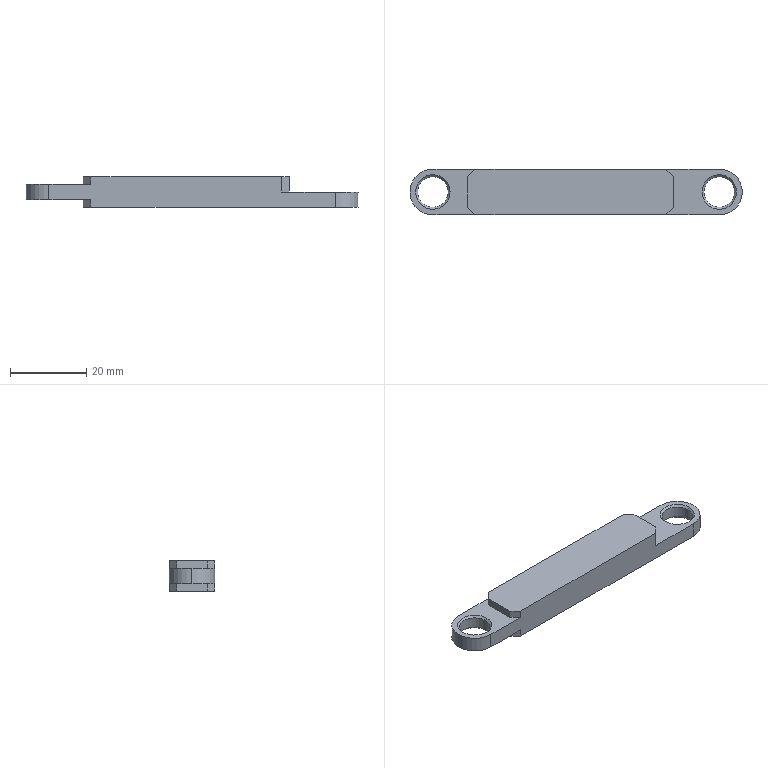Part | SolidWorks | features Chamfer 2, ICE 2, Extrusion 1 | 1 solid | 31 faces | box 87 x 12 x 8 mm | volume 6197 mm3 | plane 16 | cone 8 | cylinder 7 | commonest cylinder face diameters 8 x4 12 x3
STEP:
#1=CARTESIAN_POINT('',(33.5,0.,-0.5));
#2=VERTEX_POINT('',#1);
#3=CARTESIAN_POINT('',(41.5,0.,-0.5));
#4=VERTEX_POINT('',#3);
#5=CARTESIAN_POINT('',(37.5,0.,-0.5));
#6=DIRECTION('',(0.,0.,1.));
#7=DIRECTION('',(-1.,0.,0.));
#8=AXIS2_PLACEMENT_3D('',#5,#6,#7);
#9=CIRCLE('',#8,4.);
#10=EDGE_CURVE('',#2,#4,#9,.T.);
#11=ORIENTED_EDGE('',*,*,#10,.F.);
#12=CARTESIAN_POINT('',(33.,0.,0.));
#13=VERTEX_POINT('',#12);
#14=CARTESIAN_POINT('',(33.5,0.,-0.5));
#15=DIRECTION('',(-0.7071,0.,0.7071));
#16=VECTOR('',#15,1000.);
#17=LINE('',#14,#16);
#18=EDGE_CURVE('',#2,#13,#17,.T.);
#19=ORIENTED_EDGE('',*,*,#18,.T.);
#20=CARTESIAN_POINT('',(42.,0.,0.));
#21=VERTEX_POINT('',#20);
#22=CARTESIAN_POINT('',(37.5,0.,0.));
#23=DIRECTION('',(0.,0.,-1.));
#24=DIRECTION('',(-1.,0.,0.));
#25=AXIS2_PLACEMENT_3D('',#22,#23,#24);
#26=CIRCLE('',#25,4.5);
#27=EDGE_CURVE('',#21,#13,#26,.T.);
#28=ORIENTED_EDGE('',*,*,#27,.F.);
#29=CARTESIAN_POINT('',(41.5,0.,-0.5));
#30=DIRECTION('',(0.7071,0.,0.7071));
#31=VECTOR('',#30,1000.);
#32=LINE('',#29,#31);
#33=EDGE_CURVE('',#4,#21,#32,.T.);
#34=ORIENTED_EDGE('',*,*,#33,.F.);
#35=EDGE_LOOP('',(#11,#19,#28,#34));
#36=FACE_OUTER_BOUND('',#35,.T.);
#37=CARTESIAN_POINT('',(37.5,0.,-0.5));
#38=DIRECTION('',(0.,0.,1.));
#39=DIRECTION('',(1.,0.,0.));
#40=AXIS2_PLACEMENT_3D('',#37,#38,#39);
#41=CONICAL_SURFACE('',#40,4.,0.7854);
#42=ADVANCED_FACE('',(#36),#41,.F.);
#43=CARTESIAN_POINT('',(41.5,0.,-3.5));
#44=VERTEX_POINT('',#43);
#45=CARTESIAN_POINT('',(33.5,0.,-3.5));
#46=VERTEX_POINT('',#45);
#47=CARTESIAN_POINT('',(37.5,0.,-3.5));
#48=DIRECTION('',(0.,0.,-1.));
#49=DIRECTION('',(1.,0.,0.));
#50=AXIS2_PLACEMENT_3D('',#47,#48,#49);
#51=CIRCLE('',#50,4.);
#52=EDGE_CURVE('',#44,#46,#51,.T.);
#53=ORIENTED_EDGE('',*,*,#52,.F.);
#54=CARTESIAN_POINT('',(42.,0.,-4.));
#55=VERTEX_POINT('',#54);
#56=CARTESIAN_POINT('',(42.,0.,-4.));
#57=DIRECTION('',(0.7071,0.,-0.7071));
#58=VECTOR('',#57,1000.);
#59=LINE('',#56,#58);
#60=EDGE_CURVE('',#44,#55,#59,.T.);
#61=ORIENTED_EDGE('',*,*,#60,.T.);
#62=CARTESIAN_POINT('',(33.,0.,-4.));
#63=VERTEX_POINT('',#62);
#64=CARTESIAN_POINT('',(37.5,0.,-4.));
#65=DIRECTION('',(0.,0.,1.));
#66=DIRECTION('',(1.,0.,0.));
#67=AXIS2_PLACEMENT_3D('',#64,#65,#66);
#68=CIRCLE('',#67,4.5);
#69=EDGE_CURVE('',#63,#55,#68,.T.);
#70=ORIENTED_EDGE('',*,*,#69,.F.);
#71=CARTESIAN_POINT('',(33.,0.,-4.));
#72=DIRECTION('',(-0.7071,0.,-0.7071));
#73=VECTOR('',#72,1000.);
#74=LINE('',#71,#73);
#75=EDGE_CURVE('',#46,#63,#74,.T.);
#76=ORIENTED_EDGE('',*,*,#75,.F.);
#77=EDGE_LOOP('',(#53,#61,#70,#76));
#78=FACE_OUTER_BOUND('',#77,.T.);
#79=CARTESIAN_POINT('',(37.5,0.,-4.));
#80=DIRECTION('',(0.,0.,-1.));
#81=DIRECTION('',(-1.,0.,0.));
#82=AXIS2_PLACEMENT_3D('',#79,#80,#81);
#83=CONICAL_SURFACE('',#82,4.5,0.7854);
#84=ADVANCED_FACE('',(#78),#83,.F.);
#85=CARTESIAN_POINT('',(-41.5,0.,1.5));
#86=VERTEX_POINT('',#85);
#87=CARTESIAN_POINT('',(-33.5,0.,1.5));
#88=VERTEX_POINT('',#87);
#89=CARTESIAN_POINT('',(-37.5,0.,1.5));
#90=DIRECTION('',(0.,0.,1.));
#91=DIRECTION('',(-1.,0.,0.));
#92=AXIS2_PLACEMENT_3D('',#89,#90,#91);
#93=CIRCLE('',#92,4.);
#94=EDGE_CURVE('',#86,#88,#93,.T.);
#95=ORIENTED_EDGE('',*,*,#94,.F.);
#96=CARTESIAN_POINT('',(-42.,0.,2.));
#97=VERTEX_POINT('',#96);
#98=CARTESIAN_POINT('',(-41.5,0.,1.5));
#99=DIRECTION('',(-0.7071,0.,0.7071));
#100=VECTOR('',#99,1000.);
#101=LINE('',#98,#100);
#102=EDGE_CURVE('',#86,#97,#101,.T.);
#103=ORIENTED_EDGE('',*,*,#102,.T.);
#104=CARTESIAN_POINT('',(-33.,0.,2.));
#105=VERTEX_POINT('',#104);
#106=CARTESIAN_POINT('',(-37.5,0.,2.));
#107=DIRECTION('',(0.,0.,-1.));
#108=DIRECTION('',(-1.,0.,0.));
#109=AXIS2_PLACEMENT_3D('',#106,#107,#108);
#110=CIRCLE('',#109,4.5);
#111=EDGE_CURVE('',#105,#97,#110,.T.);
#112=ORIENTED_EDGE('',*,*,#111,.F.);
#113=CARTESIAN_POINT('',(-33.5,0.,1.5));
#114=DIRECTION('',(0.7071,0.,0.7071));
#115=VECTOR('',#114,1000.);
#116=LINE('',#113,#115);
#117=EDGE_CURVE('',#88,#105,#116,.T.);
#118=ORIENTED_EDGE('',*,*,#117,.F.);
#119=EDGE_LOOP('',(#95,#103,#112,#118));
#120=FACE_OUTER_BOUND('',#119,.T.);
#121=CARTESIAN_POINT('',(-37.5,0.,1.5));
#122=DIRECTION('',(0.,0.,1.));
#123=DIRECTION('',(1.,0.,0.));
#124=AXIS2_PLACEMENT_3D('',#121,#122,#123);
#125=CONICAL_SURFACE('',#124,4.,0.7854);
#126=ADVANCED_FACE('',(#120),#125,.F.);
#127=CARTESIAN_POINT('',(-33.5,0.,-1.5));
#128=VERTEX_POINT('',#127);
#129=CARTESIAN_POINT('',(-41.5,0.,-1.5));
#130=VERTEX_POINT('',#129);
#131=CARTESIAN_POINT('',(-37.5,0.,-1.5));
#132=DIRECTION('',(0.,0.,-1.));
#133=DIRECTION('',(1.,0.,0.));
#134=AXIS2_PLACEMENT_3D('',#131,#132,#133);
#135=CIRCLE('',#134,4.);
#136=EDGE_CURVE('',#128,#130,#135,.T.);
#137=ORIENTED_EDGE('',*,*,#136,.F.);
#138=CARTESIAN_POINT('',(-33.,0.,-2.));
#139=VERTEX_POINT('',#138);
#140=CARTESIAN_POINT('',(-33.5,0.,-1.5));
#141=DIRECTION('',(0.7071,0.,-0.7071));
#142=VECTOR('',#141,1000.);
#143=LINE('',#140,#142);
#144=EDGE_CURVE('',#128,#139,#143,.T.);
#145=ORIENTED_EDGE('',*,*,#144,.T.);
#146=CARTESIAN_POINT('',(-42.,0.,-2.));
#147=VERTEX_POINT('',#146);
#148=CARTESIAN_POINT('',(-37.5,0.,-2.));
#149=DIRECTION('',(0.,0.,1.));
#150=DIRECTION('',(1.,0.,0.));
#151=AXIS2_PLACEMENT_3D('',#148,#149,#150);
#152=CIRCLE('',#151,4.5);
#153=EDGE_CURVE('',#147,#139,#152,.T.);
#154=ORIENTED_EDGE('',*,*,#153,.F.);
#155=CARTESIAN_POINT('',(-41.5,0.,-1.5));
#156=DIRECTION('',(-0.7071,0.,-0.7071));
#157=VECTOR('',#156,1000.);
#158=LINE('',#155,#157);
#159=EDGE_CURVE('',#130,#147,#158,.T.);
#160=ORIENTED_EDGE('',*,*,#159,.F.);
#161=EDGE_LOOP('',(#137,#145,#154,#160));
#162=FACE_OUTER_BOUND('',#161,.T.);
#163=CARTESIAN_POINT('',(-37.5,0.,-1.5));
#164=DIRECTION('',(0.,0.,-1.));
#165=DIRECTION('',(-1.,0.,0.));
#166=AXIS2_PLACEMENT_3D('',#163,#164,#165);
#167=CONICAL_SURFACE('',#166,4.,0.7854);
#168=ADVANCED_FACE('',(#162),#167,.F.);
#169=ORIENTED_EDGE('',*,*,#136,.T.);
#170=CARTESIAN_POINT('',(-41.5,0.,-4.));
#171=DIRECTION('',(0.,0.,1.));
#172=VECTOR('',#171,1000.);
#173=LINE('',#170,#172);
#174=EDGE_CURVE('',#130,#86,#173,.T.);
#175=ORIENTED_EDGE('',*,*,#174,.T.);
#176=ORIENTED_EDGE('',*,*,#94,.T.);
#177=CARTESIAN_POINT('',(-33.5,0.,-4.));
#178=DIRECTION('',(0.,0.,1.));
#179=VECTOR('',#178,1000.);
#180=LINE('',#177,#179);
#181=EDGE_CURVE('',#128,#88,#180,.T.);
#182=ORIENTED_EDGE('',*,*,#181,.F.);
#183=EDGE_LOOP('',(#169,#175,#176,#182));
#184=FACE_OUTER_BOUND('',#183,.T.);
#185=CARTESIAN_POINT('',(-37.5,0.,-4.));
#186=DIRECTION('',(0.,0.,1.));
#187=DIRECTION('',(1.,0.,0.));
#188=AXIS2_PLACEMENT_3D('',#185,#186,#187);
#189=CYLINDRICAL_SURFACE('',#188,4.);
#190=ADVANCED_FACE('',(#184),#189,.F.);
#191=ORIENTED_EDGE('',*,*,#52,.T.);
#192=CARTESIAN_POINT('',(33.5,0.,-4.));
#193=DIRECTION('',(0.,0.,1.));
#194=VECTOR('',#193,1000.);
#195=LINE('',#192,#194);
#196=EDGE_CURVE('',#46,#2,#195,.T.);
#197=ORIENTED_EDGE('',*,*,#196,.T.);
#198=ORIENTED_EDGE('',*,*,#10,.T.);
#199=CARTESIAN_POINT('',(41.5,0.,-4.));
#200=DIRECTION('',(0.,0.,1.));
#201=VECTOR('',#200,1000.);
#202=LINE('',#199,#201);
#203=EDGE_CURVE('',#44,#4,#202,.T.);
#204=ORIENTED_EDGE('',*,*,#203,.F.);
#205=EDGE_LOOP('',(#191,#197,#198,#204));
#206=FACE_OUTER_BOUND('',#205,.T.);
#207=CARTESIAN_POINT('',(37.5,0.,-4.));
#208=DIRECTION('',(0.,0.,1.));
#209=DIRECTION('',(1.,0.,0.));
#210=AXIS2_PLACEMENT_3D('',#207,#208,#209);
#211=CYLINDRICAL_SURFACE('',#210,4.);
#212=ADVANCED_FACE('',(#206),#211,.F.);
#213=CARTESIAN_POINT('',(-37.5,-6.,2.));
#214=VERTEX_POINT('',#213);
#215=CARTESIAN_POINT('',(-43.5,0.,2.));
#216=VERTEX_POINT('',#215);
#217=CARTESIAN_POINT('',(-37.5,0.,2.));
#218=DIRECTION('',(0.,0.,-1.));
#219=DIRECTION('',(-1.,0.,0.));
#220=AXIS2_PLACEMENT_3D('',#217,#218,#219);
#221=CIRCLE('',#220,6.);
#222=EDGE_CURVE('',#214,#216,#221,.T.);
#223=ORIENTED_EDGE('',*,*,#222,.T.);
#224=CARTESIAN_POINT('',(-43.5,0.,-2.));
#225=VERTEX_POINT('',#224);
#226=CARTESIAN_POINT('',(-43.5,0.,4.));
#227=DIRECTION('',(0.,0.,-1.));
#228=VECTOR('',#227,1000.);
#229=LINE('',#226,#228);
#230=EDGE_CURVE('',#216,#225,#229,.T.);
#231=ORIENTED_EDGE('',*,*,#230,.T.);
#232=CARTESIAN_POINT('',(-37.5,-6.,-2.));
#233=VERTEX_POINT('',#232);
#234=CARTESIAN_POINT('',(-37.5,0.,-2.));
#235=DIRECTION('',(0.,0.,1.));
#236=DIRECTION('',(1.,0.,0.));
#237=AXIS2_PLACEMENT_3D('',#234,#235,#236);
#238=CIRCLE('',#237,6.);
#239=EDGE_CURVE('',#225,#233,#238,.T.);
#240=ORIENTED_EDGE('',*,*,#239,.T.);
#241=CARTESIAN_POINT('',(-37.5,-6.,4.));
#242=DIRECTION('',(0.,0.,-1.));
#243=VECTOR('',#242,1000.);
#244=LINE('',#241,#243);
#245=EDGE_CURVE('',#214,#233,#244,.T.);
#246=ORIENTED_EDGE('',*,*,#245,.F.);
#247=EDGE_LOOP('',(#223,#231,#240,#246));
#248=FACE_OUTER_BOUND('',#247,.T.);
#249=CARTESIAN_POINT('',(-37.5,0.,4.));
#250=DIRECTION('',(0.,0.,-1.));
#251=DIRECTION('',(-1.,0.,0.));
#252=AXIS2_PLACEMENT_3D('',#249,#250,#251);
#253=CYLINDRICAL_SURFACE('',#252,6.);
#254=ADVANCED_FACE('',(#248),#253,.T.);
#255=ORIENTED_EDGE('',*,*,#230,.F.);
#256=CARTESIAN_POINT('',(-37.5,6.,2.));
#257=VERTEX_POINT('',#256);
#258=CARTESIAN_POINT('',(-37.5,0.,2.));
#259=DIRECTION('',(0.,0.,-1.));
#260=DIRECTION('',(-1.,0.,0.));
#261=AXIS2_PLACEMENT_3D('',#258,#259,#260);
#262=CIRCLE('',#261,6.);
#263=EDGE_CURVE('',#216,#257,#262,.T.);
#264=ORIENTED_EDGE('',*,*,#263,.T.);
#265=CARTESIAN_POINT('',(-37.5,6.,-2.));
#266=VERTEX_POINT('',#265);
#267=CARTESIAN_POINT('',(-37.5,6.,4.));
#268=DIRECTION('',(0.,0.,-1.));
#269=VECTOR('',#268,1000.);
#270=LINE('',#267,#269);
#271=EDGE_CURVE('',#257,#266,#270,.T.);
#272=ORIENTED_EDGE('',*,*,#271,.T.);
#273=CARTESIAN_POINT('',(-37.5,0.,-2.));
#274=DIRECTION('',(0.,0.,1.));
#275=DIRECTION('',(1.,0.,0.));
#276=AXIS2_PLACEMENT_3D('',#273,#274,#275);
#277=CIRCLE('',#276,6.);
#278=EDGE_CURVE('',#266,#225,#277,.T.);
#279=ORIENTED_EDGE('',*,*,#278,.T.);
#280=EDGE_LOOP('',(#255,#264,#272,#279));
#281=FACE_OUTER_BOUND('',#280,.T.);
#282=CARTESIAN_POINT('',(-37.5,0.,4.));
#283=DIRECTION('',(0.,0.,-1.));
#284=DIRECTION('',(-1.,0.,0.));
#285=AXIS2_PLACEMENT_3D('',#282,#283,#284);
#286=CYLINDRICAL_SURFACE('',#285,6.);
#287=ADVANCED_FACE('',(#281),#286,.T.);
#288=CARTESIAN_POINT('',(-26.5,-6.,-2.));
#289=VERTEX_POINT('',#288);
#290=CARTESIAN_POINT('',(-43.5,-6.,-2.));
#291=DIRECTION('',(1.,0.,0.));
#292=VECTOR('',#291,1000.);
#293=LINE('',#290,#292);
#294=EDGE_CURVE('',#233,#289,#293,.T.);
#295=ORIENTED_EDGE('',*,*,#294,.T.);
#296=CARTESIAN_POINT('',(-26.5,-6.,-4.));
#297=VERTEX_POINT('',#296);
#298=CARTESIAN_POINT('',(-26.5,-6.,4.));
#299=DIRECTION('',(0.,0.,-1.));
#300=VECTOR('',#299,1000.);
#301=LINE('',#298,#300);
#302=EDGE_CURVE('',#289,#297,#301,.T.);
#303=ORIENTED_EDGE('',*,*,#302,.T.);
#304=CARTESIAN_POINT('',(37.5,-6.,-4.));
#305=VERTEX_POINT('',#304);
#306=CARTESIAN_POINT('',(-37.5,-6.,-4.));
#307=DIRECTION('',(1.,0.,0.));
#308=VECTOR('',#307,1000.);
#309=LINE('',#306,#308);
#310=EDGE_CURVE('',#297,#305,#309,.T.);
#311=ORIENTED_EDGE('',*,*,#310,.T.);
#312=CARTESIAN_POINT('',(37.5,-6.,0.));
#313=VERTEX_POINT('',#312);
#314=CARTESIAN_POINT('',(37.5,-6.,4.));
#315=DIRECTION('',(0.,0.,-1.));
#316=VECTOR('',#315,1000.);
#317=LINE('',#314,#316);
#318=EDGE_CURVE('',#313,#305,#317,.T.);
#319=ORIENTED_EDGE('',*,*,#318,.F.);
#320=CARTESIAN_POINT('',(23.5,-6.,0.));
#321=VERTEX_POINT('',#320);
#322=CARTESIAN_POINT('',(25.5,-6.,0.));
#323=DIRECTION('',(-1.,0.,0.));
#324=VECTOR('',#323,1000.);
#325=LINE('',#322,#324);
#326=EDGE_CURVE('',#313,#321,#325,.T.);
#327=ORIENTED_EDGE('',*,*,#326,.T.);
#328=CARTESIAN_POINT('',(23.5,-6.,4.));
#329=VERTEX_POINT('',#328);
#330=CARTESIAN_POINT('',(23.5,-6.,4.));
#331=DIRECTION('',(0.,0.,1.));
#332=VECTOR('',#331,1000.);
#333=LINE('',#330,#332);
#334=EDGE_CURVE('',#321,#329,#333,.T.);
#335=ORIENTED_EDGE('',*,*,#334,.T.);
#336=CARTESIAN_POINT('',(-26.5,-6.,4.));
#337=VERTEX_POINT('',#336);
#338=CARTESIAN_POINT('',(-37.5,-6.,4.));
#339=DIRECTION('',(1.,0.,0.));
#340=VECTOR('',#339,1000.);
#341=LINE('',#338,#340);
#342=EDGE_CURVE('',#337,#329,#341,.T.);
#343=ORIENTED_EDGE('',*,*,#342,.F.);
#344=CARTESIAN_POINT('',(-26.5,-6.,2.));
#345=VERTEX_POINT('',#344);
#346=CARTESIAN_POINT('',(-26.5,-6.,4.));
#347=DIRECTION('',(0.,0.,-1.));
#348=VECTOR('',#347,1000.);
#349=LINE('',#346,#348);
#350=EDGE_CURVE('',#337,#345,#349,.T.);
#351=ORIENTED_EDGE('',*,*,#350,.T.);
#352=CARTESIAN_POINT('',(-43.5,-6.,2.));
#353=DIRECTION('',(-1.,0.,0.));
#354=VECTOR('',#353,1000.);
#355=LINE('',#352,#354);
#356=EDGE_CURVE('',#345,#214,#355,.T.);
#357=ORIENTED_EDGE('',*,*,#356,.T.);
#358=ORIENTED_EDGE('',*,*,#245,.T.);
#359=EDGE_LOOP('',(#295,#303,#311,#319,#327,#335,#343,#351,#357,#358));
#360=FACE_OUTER_BOUND('',#359,.T.);
#361=CARTESIAN_POINT('',(-37.5,-6.,4.));
#362=DIRECTION('',(0.,1.,0.));
#363=DIRECTION('',(0.,0.,1.));
#364=AXIS2_PLACEMENT_3D('',#361,#362,#363);
#365=PLANE('',#364);
#366=ADVANCED_FACE('',(#360),#365,.F.);
#367=CARTESIAN_POINT('',(37.5,6.,0.));
#368=VERTEX_POINT('',#367);
#369=CARTESIAN_POINT('',(37.5,6.,-4.));
#370=VERTEX_POINT('',#369);
#371=CARTESIAN_POINT('',(37.5,6.,4.));
#372=DIRECTION('',(0.,0.,-1.));
#373=VECTOR('',#372,1000.);
#374=LINE('',#371,#373);
#375=EDGE_CURVE('',#368,#370,#374,.T.);
#376=ORIENTED_EDGE('',*,*,#375,.F.);
#377=CARTESIAN_POINT('',(37.5,0.,0.));
#378=DIRECTION('',(0.,0.,-1.));
#379=DIRECTION('',(-1.,0.,0.));
#380=AXIS2_PLACEMENT_3D('',#377,#378,#379);
#381=CIRCLE('',#380,6.);
#382=EDGE_CURVE('',#368,#313,#381,.T.);
#383=ORIENTED_EDGE('',*,*,#382,.T.);
#384=ORIENTED_EDGE('',*,*,#318,.T.);
#385=CARTESIAN_POINT('',(37.5,0.,-4.));
#386=DIRECTION('',(0.,0.,1.));
#387=DIRECTION('',(1.,0.,0.));
#388=AXIS2_PLACEMENT_3D('',#385,#386,#387);
#389=CIRCLE('',#388,6.);
#390=EDGE_CURVE('',#305,#370,#389,.T.);
#391=ORIENTED_EDGE('',*,*,#390,.T.);
#392=EDGE_LOOP('',(#376,#383,#384,#391));
#393=FACE_OUTER_BOUND('',#392,.T.);
#394=CARTESIAN_POINT('',(37.5,0.,4.));
#395=DIRECTION('',(0.,0.,-1.));
#396=DIRECTION('',(-1.,0.,0.));
#397=AXIS2_PLACEMENT_3D('',#394,#395,#396);
#398=CYLINDRICAL_SURFACE('',#397,6.);
#399=ADVANCED_FACE('',(#393),#398,.T.);
#400=CARTESIAN_POINT('',(-26.5,6.,-4.));
#401=VERTEX_POINT('',#400);
#402=CARTESIAN_POINT('',(-37.5,6.,-4.));
#403=DIRECTION('',(-1.,0.,0.));
#404=VECTOR('',#403,1000.);
#405=LINE('',#402,#404);
#406=EDGE_CURVE('',#370,#401,#405,.T.);
#407=ORIENTED_EDGE('',*,*,#406,.T.);
#408=CARTESIAN_POINT('',(-26.5,6.,-2.));
#409=VERTEX_POINT('',#408);
#410=CARTESIAN_POINT('',(-26.5,6.,4.));
#411=DIRECTION('',(0.,0.,1.));
#412=VECTOR('',#411,1000.);
#413=LINE('',#410,#412);
#414=EDGE_CURVE('',#401,#409,#413,.T.);
#415=ORIENTED_EDGE('',*,*,#414,.T.);
#416=CARTESIAN_POINT('',(-43.5,6.,-2.));
#417=DIRECTION('',(1.,0.,0.));
#418=VECTOR('',#417,1000.);
#419=LINE('',#416,#418);
#420=EDGE_CURVE('',#266,#409,#419,.T.);
#421=ORIENTED_EDGE('',*,*,#420,.F.);
#422=ORIENTED_EDGE('',*,*,#271,.F.);
#423=CARTESIAN_POINT('',(-26.5,6.,2.));
#424=VERTEX_POINT('',#423);
#425=CARTESIAN_POINT('',(-43.5,6.,2.));
#426=DIRECTION('',(-1.,0.,0.));
#427=VECTOR('',#426,1000.);
#428=LINE('',#425,#427);
#429=EDGE_CURVE('',#424,#257,#428,.T.);
#430=ORIENTED_EDGE('',*,*,#429,.F.);
#431=CARTESIAN_POINT('',(-26.5,6.,4.));
#432=VERTEX_POINT('',#431);
#433=CARTESIAN_POINT('',(-26.5,6.,4.));
#434=DIRECTION('',(0.,0.,1.));
#435=VECTOR('',#434,1000.);
#436=LINE('',#433,#435);
#437=EDGE_CURVE('',#424,#432,#436,.T.);
#438=ORIENTED_EDGE('',*,*,#437,.T.);
#439=CARTESIAN_POINT('',(23.5,6.,4.));
#440=VERTEX_POINT('',#439);
#441=CARTESIAN_POINT('',(-37.5,6.,4.));
#442=DIRECTION('',(-1.,0.,0.));
#443=VECTOR('',#442,1000.);
#444=LINE('',#441,#443);
#445=EDGE_CURVE('',#440,#432,#444,.T.);
#446=ORIENTED_EDGE('',*,*,#445,.F.);
#447=CARTESIAN_POINT('',(23.5,6.,0.));
#448=VERTEX_POINT('',#447);
#449=CARTESIAN_POINT('',(23.5,6.,4.));
#450=DIRECTION('',(0.,0.,-1.));
#451=VECTOR('',#450,1000.);
#452=LINE('',#449,#451);
#453=EDGE_CURVE('',#440,#448,#452,.T.);
#454=ORIENTED_EDGE('',*,*,#453,.T.);
#455=CARTESIAN_POINT('',(25.5,6.,0.));
#456=DIRECTION('',(-1.,0.,0.));
#457=VECTOR('',#456,1000.);
#458=LINE('',#455,#457);
#459=EDGE_CURVE('',#368,#448,#458,.T.);
#460=ORIENTED_EDGE('',*,*,#459,.F.);
#461=ORIENTED_EDGE('',*,*,#375,.T.);
#462=EDGE_LOOP('',(#407,#415,#421,#422,#430,#438,#446,#454,#460,#461));
#463=FACE_OUTER_BOUND('',#462,.T.);
#464=CARTESIAN_POINT('',(-37.5,6.,4.));
#465=DIRECTION('',(0.,-1.,0.));
#466=DIRECTION('',(0.,0.,-1.));
#467=AXIS2_PLACEMENT_3D('',#464,#465,#466);
#468=PLANE('',#467);
#469=ADVANCED_FACE('',(#463),#468,.F.);
#470=ORIENTED_EDGE('',*,*,#445,.T.);
#471=CARTESIAN_POINT('',(-28.5,4.,4.));
#472=VERTEX_POINT('',#471);
#473=CARTESIAN_POINT('',(-35.,-2.5,4.));
#474=DIRECTION('',(-0.7071,-0.7071,0.));
#475=VECTOR('',#474,1000.);
#476=LINE('',#473,#475);
#477=EDGE_CURVE('',#432,#472,#476,.T.);
#478=ORIENTED_EDGE('',*,*,#477,.T.);
#479=CARTESIAN_POINT('',(-28.5,-4.,4.));
#480=VERTEX_POINT('',#479);
#481=CARTESIAN_POINT('',(-28.5,-6.,4.));
#482=DIRECTION('',(0.,1.,0.));
#483=VECTOR('',#482,1000.);
#484=LINE('',#481,#483);
#485=EDGE_CURVE('',#480,#472,#484,.T.);
#486=ORIENTED_EDGE('',*,*,#485,.F.);
#487=CARTESIAN_POINT('',(-35.,2.5,4.));
#488=DIRECTION('',(0.7071,-0.7071,0.));
#489=VECTOR('',#488,1000.);
#490=LINE('',#487,#489);
#491=EDGE_CURVE('',#480,#337,#490,.T.);
#492=ORIENTED_EDGE('',*,*,#491,.T.);
#493=ORIENTED_EDGE('',*,*,#342,.T.);
#494=CARTESIAN_POINT('',(25.5,-4.,4.));
#495=VERTEX_POINT('',#494);
#496=CARTESIAN_POINT('',(-4.,-33.5,4.));
#497=DIRECTION('',(0.7071,0.7071,0.));
#498=VECTOR('',#497,1000.);
#499=LINE('',#496,#498);
#500=EDGE_CURVE('',#329,#495,#499,.T.);
#501=ORIENTED_EDGE('',*,*,#500,.T.);
#502=CARTESIAN_POINT('',(25.5,4.,4.));
#503=VERTEX_POINT('',#502);
#504=CARTESIAN_POINT('',(25.5,-6.,4.));
#505=DIRECTION('',(0.,1.,0.));
#506=VECTOR('',#505,1000.);
#507=LINE('',#504,#506);
#508=EDGE_CURVE('',#495,#503,#507,.T.);
#509=ORIENTED_EDGE('',*,*,#508,.T.);
#510=CARTESIAN_POINT('',(-4.,33.5,4.));
#511=DIRECTION('',(-0.7071,0.7071,0.));
#512=VECTOR('',#511,1000.);
#513=LINE('',#510,#512);
#514=EDGE_CURVE('',#503,#440,#513,.T.);
#515=ORIENTED_EDGE('',*,*,#514,.T.);
#516=EDGE_LOOP('',(#470,#478,#486,#492,#493,#501,#509,#515));
#517=FACE_OUTER_BOUND('',#516,.T.);
#518=CARTESIAN_POINT('',(-37.5,0.,4.));
#519=DIRECTION('',(0.,0.,1.));
#520=DIRECTION('',(1.,0.,0.));
#521=AXIS2_PLACEMENT_3D('',#518,#519,#520);
#522=PLANE('',#521);
#523=ADVANCED_FACE('',(#517),#522,.T.);
#524=ORIENTED_EDGE('',*,*,#69,.T.);
#525=CARTESIAN_POINT('',(37.5,0.,-4.));
#526=DIRECTION('',(0.,0.,1.));
#527=DIRECTION('',(1.,0.,0.));
#528=AXIS2_PLACEMENT_3D('',#525,#526,#527);
#529=CIRCLE('',#528,4.5);
#530=EDGE_CURVE('',#55,#63,#529,.T.);
#531=ORIENTED_EDGE('',*,*,#530,.T.);
#532=EDGE_LOOP('',(#524,#531));
#533=FACE_BOUND('',#532,.T.);
#534=CARTESIAN_POINT('',(-28.5,-4.,-4.));
#535=VERTEX_POINT('',#534);
#536=CARTESIAN_POINT('',(-28.5,4.,-4.));
#537=VERTEX_POINT('',#536);
#538=CARTESIAN_POINT('',(-28.5,-6.,-4.));
#539=DIRECTION('',(0.,1.,0.));
#540=VECTOR('',#539,1000.);
#541=LINE('',#538,#540);
#542=EDGE_CURVE('',#535,#537,#541,.T.);
#543=ORIENTED_EDGE('',*,*,#542,.T.);
#544=CARTESIAN_POINT('',(-28.5,4.,-4.));
#545=DIRECTION('',(0.7071,0.7071,0.));
#546=VECTOR('',#545,1000.);
#547=LINE('',#544,#546);
#548=EDGE_CURVE('',#537,#401,#547,.T.);
#549=ORIENTED_EDGE('',*,*,#548,.T.);
#550=ORIENTED_EDGE('',*,*,#406,.F.);
#551=ORIENTED_EDGE('',*,*,#390,.F.);
#552=ORIENTED_EDGE('',*,*,#310,.F.);
#553=CARTESIAN_POINT('',(-26.5,-6.,-4.));
#554=DIRECTION('',(-0.7071,0.7071,0.));
#555=VECTOR('',#554,1000.);
#556=LINE('',#553,#555);
#557=EDGE_CURVE('',#297,#535,#556,.T.);
#558=ORIENTED_EDGE('',*,*,#557,.T.);
#559=EDGE_LOOP('',(#543,#549,#550,#551,#552,#558));
#560=FACE_OUTER_BOUND('',#559,.T.);
#561=CARTESIAN_POINT('',(-37.5,0.,-4.));
#562=DIRECTION('',(0.,0.,1.));
#563=DIRECTION('',(1.,0.,0.));
#564=AXIS2_PLACEMENT_3D('',#561,#562,#563);
#565=PLANE('',#564);
#566=ADVANCED_FACE('',(#533,#560),#565,.F.);
#567=ORIENTED_EDGE('',*,*,#196,.F.);
#568=CARTESIAN_POINT('',(37.5,0.,-3.5));
#569=DIRECTION('',(0.,0.,-1.));
#570=DIRECTION('',(1.,0.,0.));
#571=AXIS2_PLACEMENT_3D('',#568,#569,#570);
#572=CIRCLE('',#571,4.);
#573=EDGE_CURVE('',#46,#44,#572,.T.);
#574=ORIENTED_EDGE('',*,*,#573,.T.);
#575=ORIENTED_EDGE('',*,*,#203,.T.);
#576=CARTESIAN_POINT('',(37.5,0.,-0.5));
#577=DIRECTION('',(0.,0.,1.));
#578=DIRECTION('',(-1.,0.,0.));
#579=AXIS2_PLACEMENT_3D('',#576,#577,#578);
#580=CIRCLE('',#579,4.);
#581=EDGE_CURVE('',#4,#2,#580,.T.);
#582=ORIENTED_EDGE('',*,*,#581,.T.);
#583=EDGE_LOOP('',(#567,#574,#575,#582));
#584=FACE_OUTER_BOUND('',#583,.T.);
#585=CARTESIAN_POINT('',(37.5,0.,-4.));
#586=DIRECTION('',(0.,0.,1.));
#587=DIRECTION('',(1.,0.,0.));
#588=AXIS2_PLACEMENT_3D('',#585,#586,#587);
#589=CYLINDRICAL_SURFACE('',#588,4.);
#590=ADVANCED_FACE('',(#584),#589,.F.);
#591=ORIENTED_EDGE('',*,*,#174,.F.);
#592=CARTESIAN_POINT('',(-37.5,0.,-1.5));
#593=DIRECTION('',(0.,0.,-1.));
#594=DIRECTION('',(1.,0.,0.));
#595=AXIS2_PLACEMENT_3D('',#592,#593,#594);
#596=CIRCLE('',#595,4.);
#597=EDGE_CURVE('',#130,#128,#596,.T.);
#598=ORIENTED_EDGE('',*,*,#597,.T.);
#599=ORIENTED_EDGE('',*,*,#181,.T.);
#600=CARTESIAN_POINT('',(-37.5,0.,1.5));
#601=DIRECTION('',(0.,0.,1.));
#602=DIRECTION('',(-1.,0.,0.));
#603=AXIS2_PLACEMENT_3D('',#600,#601,#602);
#604=CIRCLE('',#603,4.);
#605=EDGE_CURVE('',#88,#86,#604,.T.);
#606=ORIENTED_EDGE('',*,*,#605,.T.);
#607=EDGE_LOOP('',(#591,#598,#599,#606));
#608=FACE_OUTER_BOUND('',#607,.T.);
#609=CARTESIAN_POINT('',(-37.5,0.,-4.));
#610=DIRECTION('',(0.,0.,1.));
#611=DIRECTION('',(1.,0.,0.));
#612=AXIS2_PLACEMENT_3D('',#609,#610,#611);
#613=CYLINDRICAL_SURFACE('',#612,4.);
#614=ADVANCED_FACE('',(#608),#613,.F.);
#615=ORIENTED_EDGE('',*,*,#27,.T.);
#616=CARTESIAN_POINT('',(37.5,0.,0.));
#617=DIRECTION('',(0.,0.,-1.));
#618=DIRECTION('',(-1.,0.,0.));
#619=AXIS2_PLACEMENT_3D('',#616,#617,#618);
#620=CIRCLE('',#619,4.5);
#621=EDGE_CURVE('',#13,#21,#620,.T.);
#622=ORIENTED_EDGE('',*,*,#621,.T.);
#623=EDGE_LOOP('',(#615,#622));
#624=FACE_BOUND('',#623,.T.);
#625=ORIENTED_EDGE('',*,*,#459,.T.);
#626=CARTESIAN_POINT('',(25.5,4.,0.));
#627=VERTEX_POINT('',#626);
#628=CARTESIAN_POINT('',(30.5,-1.,0.));
#629=DIRECTION('',(0.7071,-0.7071,0.));
#630=VECTOR('',#629,1000.);
#631=LINE('',#628,#630);
#632=EDGE_CURVE('',#448,#627,#631,.T.);
#633=ORIENTED_EDGE('',*,*,#632,.T.);
#634=CARTESIAN_POINT('',(25.5,-4.,0.));
#635=VERTEX_POINT('',#634);
#636=CARTESIAN_POINT('',(25.5,-6.,0.));
#637=DIRECTION('',(0.,1.,0.));
#638=VECTOR('',#637,1000.);
#639=LINE('',#636,#638);
#640=EDGE_CURVE('',#635,#627,#639,.T.);
#641=ORIENTED_EDGE('',*,*,#640,.F.);
#642=CARTESIAN_POINT('',(24.5,-5.,0.));
#643=DIRECTION('',(-0.7071,-0.7071,0.));
#644=VECTOR('',#643,1000.);
#645=LINE('',#642,#644);
#646=EDGE_CURVE('',#635,#321,#645,.T.);
#647=ORIENTED_EDGE('',*,*,#646,.T.);
#648=ORIENTED_EDGE('',*,*,#326,.F.);
#649=ORIENTED_EDGE('',*,*,#382,.F.);
#650=EDGE_LOOP('',(#625,#633,#641,#647,#648,#649));
#651=FACE_OUTER_BOUND('',#650,.T.);
#652=CARTESIAN_POINT('',(25.5,-6.,0.));
#653=DIRECTION('',(0.,0.,-1.));
#654=DIRECTION('',(-1.,0.,0.));
#655=AXIS2_PLACEMENT_3D('',#652,#653,#654);
#656=PLANE('',#655);
#657=ADVANCED_FACE('',(#624,#651),#656,.F.);
#658=ORIENTED_EDGE('',*,*,#640,.T.);
#659=CARTESIAN_POINT('',(25.5,4.,4.));
#660=DIRECTION('',(0.,0.,1.));
#661=VECTOR('',#660,1000.);
#662=LINE('',#659,#661);
#663=EDGE_CURVE('',#627,#503,#662,.T.);
#664=ORIENTED_EDGE('',*,*,#663,.T.);
#665=ORIENTED_EDGE('',*,*,#508,.F.);
#666=CARTESIAN_POINT('',(25.5,-4.,4.));
#667=DIRECTION('',(0.,0.,-1.));
#668=VECTOR('',#667,1000.);
#669=LINE('',#666,#668);
#670=EDGE_CURVE('',#495,#635,#669,.T.);
#671=ORIENTED_EDGE('',*,*,#670,.T.);
#672=EDGE_LOOP('',(#658,#664,#665,#671));
#673=FACE_OUTER_BOUND('',#672,.T.);
#674=CARTESIAN_POINT('',(25.5,-6.,4.));
#675=DIRECTION('',(-1.,0.,0.));
#676=DIRECTION('',(0.,0.,1.));
#677=AXIS2_PLACEMENT_3D('',#674,#675,#676);
#678=PLANE('',#677);
#679=ADVANCED_FACE('',(#673),#678,.F.);
#680=ORIENTED_EDGE('',*,*,#111,.T.);
#681=CARTESIAN_POINT('',(-37.5,0.,2.));
#682=DIRECTION('',(0.,0.,-1.));
#683=DIRECTION('',(-1.,0.,0.));
#684=AXIS2_PLACEMENT_3D('',#681,#682,#683);
#685=CIRCLE('',#684,4.5);
#686=EDGE_CURVE('',#97,#105,#685,.T.);
#687=ORIENTED_EDGE('',*,*,#686,.T.);
#688=EDGE_LOOP('',(#680,#687));
#689=FACE_BOUND('',#688,.T.);
#690=ORIENTED_EDGE('',*,*,#222,.F.);
#691=ORIENTED_EDGE('',*,*,#356,.F.);
#692=CARTESIAN_POINT('',(-28.5,-4.,2.));
#693=VERTEX_POINT('',#692);
#694=CARTESIAN_POINT('',(-35.,2.5,2.));
#695=DIRECTION('',(-0.7071,0.7071,0.));
#696=VECTOR('',#695,1000.);
#697=LINE('',#694,#696);
#698=EDGE_CURVE('',#345,#693,#697,.T.);
#699=ORIENTED_EDGE('',*,*,#698,.T.);
#700=CARTESIAN_POINT('',(-28.5,4.,2.));
#701=VERTEX_POINT('',#700);
#702=CARTESIAN_POINT('',(-28.5,-6.,2.));
#703=DIRECTION('',(0.,1.,0.));
#704=VECTOR('',#703,1000.);
#705=LINE('',#702,#704);
#706=EDGE_CURVE('',#693,#701,#705,.T.);
#707=ORIENTED_EDGE('',*,*,#706,.T.);
#708=CARTESIAN_POINT('',(-41.,-8.5,2.));
#709=DIRECTION('',(0.7071,0.7071,0.));
#710=VECTOR('',#709,1000.);
#711=LINE('',#708,#710);
#712=EDGE_CURVE('',#701,#424,#711,.T.);
#713=ORIENTED_EDGE('',*,*,#712,.T.);
#714=ORIENTED_EDGE('',*,*,#429,.T.);
#715=ORIENTED_EDGE('',*,*,#263,.F.);
#716=EDGE_LOOP('',(#690,#691,#699,#707,#713,#714,#715));
#717=FACE_OUTER_BOUND('',#716,.T.);
#718=CARTESIAN_POINT('',(-43.5,-6.,2.));
#719=DIRECTION('',(0.,0.,-1.));
#720=DIRECTION('',(-1.,0.,0.));
#721=AXIS2_PLACEMENT_3D('',#718,#719,#720);
#722=PLANE('',#721);
#723=ADVANCED_FACE('',(#689,#717),#722,.F.);
#724=ORIENTED_EDGE('',*,*,#485,.T.);
#725=CARTESIAN_POINT('',(-28.5,4.,4.));
#726=DIRECTION('',(0.,0.,-1.));
#727=VECTOR('',#726,1000.);
#728=LINE('',#725,#727);
#729=EDGE_CURVE('',#472,#701,#728,.T.);
#730=ORIENTED_EDGE('',*,*,#729,.T.);
#731=ORIENTED_EDGE('',*,*,#706,.F.);
#732=CARTESIAN_POINT('',(-28.5,-4.,4.));
#733=DIRECTION('',(0.,0.,1.));
#734=VECTOR('',#733,1000.);
#735=LINE('',#732,#734);
#736=EDGE_CURVE('',#693,#480,#735,.T.);
#737=ORIENTED_EDGE('',*,*,#736,.T.);
#738=EDGE_LOOP('',(#724,#730,#731,#737));
#739=FACE_OUTER_BOUND('',#738,.T.);
#740=CARTESIAN_POINT('',(-28.5,-6.,4.));
#741=DIRECTION('',(1.,0.,0.));
#742=DIRECTION('',(0.,0.,-1.));
#743=AXIS2_PLACEMENT_3D('',#740,#741,#742);
#744=PLANE('',#743);
#745=ADVANCED_FACE('',(#739),#744,.F.);
#746=ORIENTED_EDGE('',*,*,#153,.T.);
#747=CARTESIAN_POINT('',(-37.5,0.,-2.));
#748=DIRECTION('',(0.,0.,1.));
#749=DIRECTION('',(1.,0.,0.));
#750=AXIS2_PLACEMENT_3D('',#747,#748,#749);
#751=CIRCLE('',#750,4.5);
#752=EDGE_CURVE('',#139,#147,#751,.T.);
#753=ORIENTED_EDGE('',*,*,#752,.T.);
#754=EDGE_LOOP('',(#746,#753));
#755=FACE_BOUND('',#754,.T.);
#756=ORIENTED_EDGE('',*,*,#420,.T.);
#757=CARTESIAN_POINT('',(-28.5,4.,-2.));
#758=VERTEX_POINT('',#757);
#759=CARTESIAN_POINT('',(-41.,-8.5,-2.));
#760=DIRECTION('',(-0.7071,-0.7071,0.));
#761=VECTOR('',#760,1000.);
#762=LINE('',#759,#761);
#763=EDGE_CURVE('',#409,#758,#762,.T.);
#764=ORIENTED_EDGE('',*,*,#763,.T.);
#765=CARTESIAN_POINT('',(-28.5,-4.,-2.));
#766=VERTEX_POINT('',#765);
#767=CARTESIAN_POINT('',(-28.5,-6.,-2.));
#768=DIRECTION('',(0.,1.,0.));
#769=VECTOR('',#768,1000.);
#770=LINE('',#767,#769);
#771=EDGE_CURVE('',#766,#758,#770,.T.);
#772=ORIENTED_EDGE('',*,*,#771,.F.);
#773=CARTESIAN_POINT('',(-35.,2.5,-2.));
#774=DIRECTION('',(0.7071,-0.7071,0.));
#775=VECTOR('',#774,1000.);
#776=LINE('',#773,#775);
#777=EDGE_CURVE('',#766,#289,#776,.T.);
#778=ORIENTED_EDGE('',*,*,#777,.T.);
#779=ORIENTED_EDGE('',*,*,#294,.F.);
#780=ORIENTED_EDGE('',*,*,#239,.F.);
#781=ORIENTED_EDGE('',*,*,#278,.F.);
#782=EDGE_LOOP('',(#756,#764,#772,#778,#779,#780,#781));
#783=FACE_OUTER_BOUND('',#782,.T.);
#784=CARTESIAN_POINT('',(-43.5,-6.,-2.));
#785=DIRECTION('',(0.,0.,1.));
#786=DIRECTION('',(1.,0.,0.));
#787=AXIS2_PLACEMENT_3D('',#784,#785,#786);
#788=PLANE('',#787);
#789=ADVANCED_FACE('',(#755,#783),#788,.F.);
#790=ORIENTED_EDGE('',*,*,#771,.T.);
#791=CARTESIAN_POINT('',(-28.5,4.,-4.));
#792=DIRECTION('',(0.,0.,-1.));
#793=VECTOR('',#792,1000.);
#794=LINE('',#791,#793);
#795=EDGE_CURVE('',#758,#537,#794,.T.);
#796=ORIENTED_EDGE('',*,*,#795,.T.);
#797=ORIENTED_EDGE('',*,*,#542,.F.);
#798=CARTESIAN_POINT('',(-28.5,-4.,-4.));
#799=DIRECTION('',(0.,0.,1.));
#800=VECTOR('',#799,1000.);
#801=LINE('',#798,#800);
#802=EDGE_CURVE('',#535,#766,#801,.T.);
#803=ORIENTED_EDGE('',*,*,#802,.T.);
#804=EDGE_LOOP('',(#790,#796,#797,#803));
#805=FACE_OUTER_BOUND('',#804,.T.);
#806=CARTESIAN_POINT('',(-28.5,-6.,-4.));
#807=DIRECTION('',(1.,0.,0.));
#808=DIRECTION('',(0.,0.,-1.));
#809=AXIS2_PLACEMENT_3D('',#806,#807,#808);
#810=PLANE('',#809);
#811=ADVANCED_FACE('',(#805),#810,.F.);
#812=ORIENTED_EDGE('',*,*,#763,.F.);
#813=ORIENTED_EDGE('',*,*,#414,.F.);
#814=ORIENTED_EDGE('',*,*,#548,.F.);
#815=ORIENTED_EDGE('',*,*,#795,.F.);
#816=EDGE_LOOP('',(#812,#813,#814,#815));
#817=FACE_OUTER_BOUND('',#816,.T.);
#818=CARTESIAN_POINT('',(-28.5,4.,-4.));
#819=DIRECTION('',(0.7071,-0.7071,0.));
#820=DIRECTION('',(0.,0.,-1.));
#821=AXIS2_PLACEMENT_3D('',#818,#819,#820);
#822=PLANE('',#821);
#823=ADVANCED_FACE('',(#817),#822,.F.);
#824=ORIENTED_EDGE('',*,*,#777,.F.);
#825=ORIENTED_EDGE('',*,*,#802,.F.);
#826=ORIENTED_EDGE('',*,*,#557,.F.);
#827=ORIENTED_EDGE('',*,*,#302,.F.);
#828=EDGE_LOOP('',(#824,#825,#826,#827));
#829=FACE_OUTER_BOUND('',#828,.T.);
#830=CARTESIAN_POINT('',(-26.5,-6.,4.));
#831=DIRECTION('',(0.7071,0.7071,0.));
#832=DIRECTION('',(0.,0.,-1.));
#833=AXIS2_PLACEMENT_3D('',#830,#831,#832);
#834=PLANE('',#833);
#835=ADVANCED_FACE('',(#829),#834,.F.);
#836=ORIENTED_EDGE('',*,*,#477,.F.);
#837=ORIENTED_EDGE('',*,*,#437,.F.);
#838=ORIENTED_EDGE('',*,*,#712,.F.);
#839=ORIENTED_EDGE('',*,*,#729,.F.);
#840=EDGE_LOOP('',(#836,#837,#838,#839));
#841=FACE_OUTER_BOUND('',#840,.T.);
#842=CARTESIAN_POINT('',(-28.5,4.,4.));
#843=DIRECTION('',(0.7071,-0.7071,0.));
#844=DIRECTION('',(0.,0.,-1.));
#845=AXIS2_PLACEMENT_3D('',#842,#843,#844);
#846=PLANE('',#845);
#847=ADVANCED_FACE('',(#841),#846,.F.);
#848=ORIENTED_EDGE('',*,*,#491,.F.);
#849=ORIENTED_EDGE('',*,*,#736,.F.);
#850=ORIENTED_EDGE('',*,*,#698,.F.);
#851=ORIENTED_EDGE('',*,*,#350,.F.);
#852=EDGE_LOOP('',(#848,#849,#850,#851));
#853=FACE_OUTER_BOUND('',#852,.T.);
#854=CARTESIAN_POINT('',(-26.5,-6.,4.));
#855=DIRECTION('',(0.7071,0.7071,0.));
#856=DIRECTION('',(0.,0.,-1.));
#857=AXIS2_PLACEMENT_3D('',#854,#855,#856);
#858=PLANE('',#857);
#859=ADVANCED_FACE('',(#853),#858,.F.);
#860=ORIENTED_EDGE('',*,*,#632,.F.);
#861=ORIENTED_EDGE('',*,*,#453,.F.);
#862=ORIENTED_EDGE('',*,*,#514,.F.);
#863=ORIENTED_EDGE('',*,*,#663,.F.);
#864=EDGE_LOOP('',(#860,#861,#862,#863));
#865=FACE_OUTER_BOUND('',#864,.T.);
#866=CARTESIAN_POINT('',(25.5,4.,4.));
#867=DIRECTION('',(-0.7071,-0.7071,0.));
#868=DIRECTION('',(0.,0.,1.));
#869=AXIS2_PLACEMENT_3D('',#866,#867,#868);
#870=PLANE('',#869);
#871=ADVANCED_FACE('',(#865),#870,.F.);
#872=ORIENTED_EDGE('',*,*,#646,.F.);
#873=ORIENTED_EDGE('',*,*,#670,.F.);
#874=ORIENTED_EDGE('',*,*,#500,.F.);
#875=ORIENTED_EDGE('',*,*,#334,.F.);
#876=EDGE_LOOP('',(#872,#873,#874,#875));
#877=FACE_OUTER_BOUND('',#876,.T.);
#878=CARTESIAN_POINT('',(23.5,-6.,4.));
#879=DIRECTION('',(-0.7071,0.7071,0.));
#880=DIRECTION('',(0.,0.,1.));
#881=AXIS2_PLACEMENT_3D('',#878,#879,#880);
#882=PLANE('',#881);
#883=ADVANCED_FACE('',(#877),#882,.F.);
#884=ORIENTED_EDGE('',*,*,#144,.F.);
#885=ORIENTED_EDGE('',*,*,#597,.F.);
#886=ORIENTED_EDGE('',*,*,#159,.T.);
#887=ORIENTED_EDGE('',*,*,#752,.F.);
#888=EDGE_LOOP('',(#884,#885,#886,#887));
#889=FACE_OUTER_BOUND('',#888,.T.);
#890=CARTESIAN_POINT('',(-37.5,0.,-1.5));
#891=DIRECTION('',(0.,0.,-1.));
#892=DIRECTION('',(-1.,0.,0.));
#893=AXIS2_PLACEMENT_3D('',#890,#891,#892);
#894=CONICAL_SURFACE('',#893,4.,0.7854);
#895=ADVANCED_FACE('',(#889),#894,.F.);
#896=ORIENTED_EDGE('',*,*,#102,.F.);
#897=ORIENTED_EDGE('',*,*,#605,.F.);
#898=ORIENTED_EDGE('',*,*,#117,.T.);
#899=ORIENTED_EDGE('',*,*,#686,.F.);
#900=EDGE_LOOP('',(#896,#897,#898,#899));
#901=FACE_OUTER_BOUND('',#900,.T.);
#902=CARTESIAN_POINT('',(-37.5,0.,1.5));
#903=DIRECTION('',(0.,0.,1.));
#904=DIRECTION('',(1.,0.,0.));
#905=AXIS2_PLACEMENT_3D('',#902,#903,#904);
#906=CONICAL_SURFACE('',#905,4.,0.7854);
#907=ADVANCED_FACE('',(#901),#906,.F.);
#908=ORIENTED_EDGE('',*,*,#60,.F.);
#909=ORIENTED_EDGE('',*,*,#573,.F.);
#910=ORIENTED_EDGE('',*,*,#75,.T.);
#911=ORIENTED_EDGE('',*,*,#530,.F.);
#912=EDGE_LOOP('',(#908,#909,#910,#911));
#913=FACE_OUTER_BOUND('',#912,.T.);
#914=CARTESIAN_POINT('',(37.5,0.,-4.));
#915=DIRECTION('',(0.,0.,-1.));
#916=DIRECTION('',(-1.,0.,0.));
#917=AXIS2_PLACEMENT_3D('',#914,#915,#916);
#918=CONICAL_SURFACE('',#917,4.5,0.7854);
#919=ADVANCED_FACE('',(#913),#918,.F.);
#920=ORIENTED_EDGE('',*,*,#18,.F.);
#921=ORIENTED_EDGE('',*,*,#581,.F.);
#922=ORIENTED_EDGE('',*,*,#33,.T.);
#923=ORIENTED_EDGE('',*,*,#621,.F.);
#924=EDGE_LOOP('',(#920,#921,#922,#923));
#925=FACE_OUTER_BOUND('',#924,.T.);
#926=CARTESIAN_POINT('',(37.5,0.,-0.5));
#927=DIRECTION('',(0.,0.,1.));
#928=DIRECTION('',(1.,0.,0.));
#929=AXIS2_PLACEMENT_3D('',#926,#927,#928);
#930=CONICAL_SURFACE('',#929,4.,0.7854);
#931=ADVANCED_FACE('',(#925),#930,.F.);
#932=CLOSED_SHELL('',(#42,#84,#126,#168,#190,#212,#254,#287,#366,#399,#469,#523,#566,#590,#614,#657,#679,#723,#745,#789,#811,#823,#835,#847,#859,#871,#883,#895,#907,#919,#931));
#933=MANIFOLD_SOLID_BREP('',#932);
#934=CARTESIAN_POINT('',(0.,0.,0.));
#935=DIRECTION('',(0.,0.,1.));
#936=DIRECTION('',(1.,0.,0.));
#937=AXIS2_PLACEMENT_3D('',#934,#935,#936);
#938=(LENGTH_UNIT()NAMED_UNIT(*)SI_UNIT(.MILLI.,.METRE.));
#939=UNCERTAINTY_MEASURE_WITH_UNIT(LENGTH_MEASURE(0.00001),#938,'','');
#940=(NAMED_UNIT(*)PLANE_ANGLE_UNIT()SI_UNIT($,.RADIAN.));
#941=(NAMED_UNIT(*)SI_UNIT($,.STERADIAN.)SOLID_ANGLE_UNIT());
#942=(GEOMETRIC_REPRESENTATION_CONTEXT(3)GLOBAL_UNCERTAINTY_ASSIGNED_CONTEXT((#939))GLOBAL_UNIT_ASSIGNED_CONTEXT((#938,#940,#941))REPRESENTATION_CONTEXT('',''));
#943=ADVANCED_BREP_SHAPE_REPRESENTATION('',(#933,#937),#942);